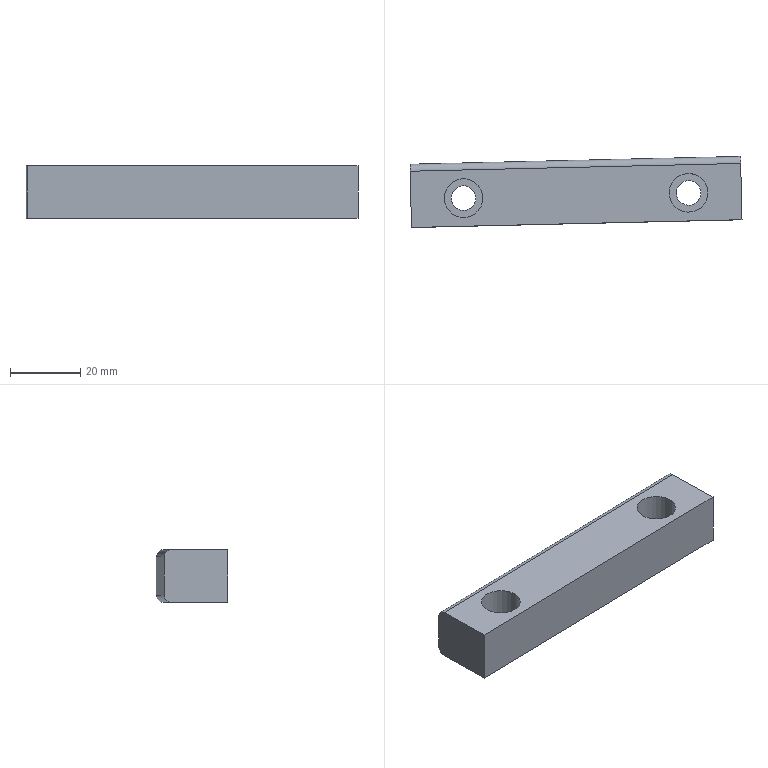Part | NX | features solid 2 | 1 solid | 14 faces | box 94.397 x 20.206 x 15 mm | volume 23046 mm3 | plane 8 | cylinder 6 | commonest cylinder face diameters 4 x2 7 x2 11 x2
STEP:
#1=CARTESIAN_POINT('',(641.92,-127.62,-12.));
#2=VERTEX_POINT('',#1);
#3=CARTESIAN_POINT('',(641.544,-111.625,-12.));
#4=VERTEX_POINT('',#3);
#5=CARTESIAN_POINT('',(641.732,-119.622,-12.));
#6=DIRECTION('',(-0.02352,0.9997,0.));
#7=VECTOR('',#6,1000.);
#8=LINE('',#5,#7);
#9=EDGE_CURVE('',#2,#4,#8,.T.);
#10=ORIENTED_EDGE('',*,*,#9,.T.);
#11=CARTESIAN_POINT('',(735.518,-109.413,-12.));
#12=VERTEX_POINT('',#11);
#13=CARTESIAN_POINT('',(735.518,-109.413,-12.));
#14=DIRECTION('',(0.9997,0.02352,0.));
#15=VECTOR('',#14,1000.);
#16=LINE('',#13,#15);
#17=EDGE_CURVE('',#4,#12,#16,.T.);
#18=ORIENTED_EDGE('',*,*,#17,.T.);
#19=CARTESIAN_POINT('',(735.894,-125.409,-12.));
#20=VERTEX_POINT('',#19);
#21=CARTESIAN_POINT('',(735.706,-117.411,-12.));
#22=DIRECTION('',(-0.02352,0.9997,0.));
#23=VECTOR('',#22,1000.);
#24=LINE('',#21,#23);
#25=EDGE_CURVE('',#20,#12,#24,.T.);
#26=ORIENTED_EDGE('',*,*,#25,.F.);
#27=CARTESIAN_POINT('',(735.894,-125.409,-12.));
#28=DIRECTION('',(0.9997,0.02352,0.));
#29=VECTOR('',#28,1000.);
#30=LINE('',#27,#29);
#31=EDGE_CURVE('',#2,#20,#30,.T.);
#32=ORIENTED_EDGE('',*,*,#31,.F.);
#33=EDGE_LOOP('',(#10,#18,#26,#32));
#34=FACE_BOUND('',#33,.T.);
#35=CARTESIAN_POINT('',(660.228,-119.27,-12.));
#36=VERTEX_POINT('',#35);
#37=CARTESIAN_POINT('',(656.728,-119.27,-12.));
#38=DIRECTION('',(0.,0.,1.));
#39=DIRECTION('',(1.,0.,0.));
#40=AXIS2_PLACEMENT_3D('',#37,#38,#39);
#41=CIRCLE('',#40,3.5);
#42=EDGE_CURVE('',#36,#36,#41,.T.);
#43=ORIENTED_EDGE('',*,*,#42,.T.);
#44=EDGE_LOOP('',(#43));
#45=FACE_BOUND('',#44,.T.);
#46=CARTESIAN_POINT('',(717.214,-117.929,-12.));
#47=VERTEX_POINT('',#46);
#48=CARTESIAN_POINT('',(720.71,-117.764,-12.));
#49=DIRECTION('',(0.,0.,-1.));
#50=DIRECTION('',(-0.9989,-0.04703,0.));
#51=AXIS2_PLACEMENT_3D('',#48,#49,#50);
#52=CIRCLE('',#51,3.5);
#53=EDGE_CURVE('',#47,#47,#52,.T.);
#54=ORIENTED_EDGE('',*,*,#53,.F.);
#55=EDGE_LOOP('',(#54));
#56=FACE_BOUND('',#55,.T.);
#57=CARTESIAN_POINT('',(735.706,-117.411,-12.));
#58=DIRECTION('',(0.,0.,1.));
#59=DIRECTION('',(1.,0.,0.));
#60=AXIS2_PLACEMENT_3D('',#57,#58,#59);
#61=PLANE('',#60);
#62=ADVANCED_FACE('',(#34,#45,#56),#61,.F.);
#63=CARTESIAN_POINT('',(735.894,-125.409,3.));
#64=VERTEX_POINT('',#63);
#65=CARTESIAN_POINT('',(735.518,-109.413,3.));
#66=VERTEX_POINT('',#65);
#67=CARTESIAN_POINT('',(735.706,-117.411,3.));
#68=DIRECTION('',(-0.02352,0.9997,0.));
#69=VECTOR('',#68,1000.);
#70=LINE('',#67,#69);
#71=EDGE_CURVE('',#64,#66,#70,.T.);
#72=ORIENTED_EDGE('',*,*,#71,.T.);
#73=CARTESIAN_POINT('',(641.544,-111.625,3.));
#74=VERTEX_POINT('',#73);
#75=CARTESIAN_POINT('',(735.518,-109.413,3.));
#76=DIRECTION('',(-0.9997,-0.02352,0.));
#77=VECTOR('',#76,1000.);
#78=LINE('',#75,#77);
#79=EDGE_CURVE('',#66,#74,#78,.T.);
#80=ORIENTED_EDGE('',*,*,#79,.T.);
#81=CARTESIAN_POINT('',(641.92,-127.62,3.));
#82=VERTEX_POINT('',#81);
#83=CARTESIAN_POINT('',(641.732,-119.622,3.));
#84=DIRECTION('',(-0.02352,0.9997,0.));
#85=VECTOR('',#84,1000.);
#86=LINE('',#83,#85);
#87=EDGE_CURVE('',#82,#74,#86,.T.);
#88=ORIENTED_EDGE('',*,*,#87,.F.);
#89=CARTESIAN_POINT('',(735.894,-125.409,3.));
#90=DIRECTION('',(-0.9997,-0.02352,0.));
#91=VECTOR('',#90,1000.);
#92=LINE('',#89,#91);
#93=EDGE_CURVE('',#64,#82,#92,.T.);
#94=ORIENTED_EDGE('',*,*,#93,.F.);
#95=EDGE_LOOP('',(#72,#80,#88,#94));
#96=FACE_BOUND('',#95,.T.);
#97=CARTESIAN_POINT('',(662.228,-119.27,3.));
#98=VERTEX_POINT('',#97);
#99=CARTESIAN_POINT('',(656.728,-119.27,3.));
#100=DIRECTION('',(0.,0.,-1.));
#101=DIRECTION('',(1.,0.,0.));
#102=AXIS2_PLACEMENT_3D('',#99,#100,#101);
#103=CIRCLE('',#102,5.5);
#104=EDGE_CURVE('',#98,#98,#103,.T.);
#105=ORIENTED_EDGE('',*,*,#104,.T.);
#106=EDGE_LOOP('',(#105));
#107=FACE_BOUND('',#106,.T.);
#108=CARTESIAN_POINT('',(715.216,-118.023,3.));
#109=VERTEX_POINT('',#108);
#110=CARTESIAN_POINT('',(720.71,-117.764,3.));
#111=DIRECTION('',(0.,0.,1.));
#112=DIRECTION('',(-0.9989,-0.04703,0.));
#113=AXIS2_PLACEMENT_3D('',#110,#111,#112);
#114=CIRCLE('',#113,5.5);
#115=EDGE_CURVE('',#109,#109,#114,.T.);
#116=ORIENTED_EDGE('',*,*,#115,.F.);
#117=EDGE_LOOP('',(#116));
#118=FACE_BOUND('',#117,.T.);
#119=CARTESIAN_POINT('',(735.706,-117.411,3.));
#120=DIRECTION('',(0.,0.,-1.));
#121=DIRECTION('',(-1.,0.,0.));
#122=AXIS2_PLACEMENT_3D('',#119,#120,#121);
#123=PLANE('',#122);
#124=ADVANCED_FACE('',(#96,#107,#118),#123,.F.);
#125=CARTESIAN_POINT('',(641.496,-109.625,1.));
#126=VERTEX_POINT('',#125);
#127=CARTESIAN_POINT('',(641.496,-109.625,-10.));
#128=VERTEX_POINT('',#127);
#129=CARTESIAN_POINT('',(641.496,-109.625,50.));
#130=DIRECTION('',(0.,0.,-1.));
#131=VECTOR('',#130,1000.);
#132=LINE('',#129,#131);
#133=EDGE_CURVE('',#126,#128,#132,.T.);
#134=ORIENTED_EDGE('',*,*,#133,.T.);
#135=CARTESIAN_POINT('',(641.544,-111.625,-10.));
#136=DIRECTION('',(0.9997,0.02352,0.));
#137=DIRECTION('',(-0.02352,0.9997,0.));
#138=AXIS2_PLACEMENT_3D('',#135,#136,#137);
#139=CIRCLE('',#138,2.);
#140=EDGE_CURVE('',#128,#4,#139,.F.);
#141=ORIENTED_EDGE('',*,*,#140,.T.);
#142=ORIENTED_EDGE('',*,*,#9,.F.);
#143=CARTESIAN_POINT('',(641.92,-127.62,50.));
#144=DIRECTION('',(0.,0.,-1.));
#145=VECTOR('',#144,1000.);
#146=LINE('',#143,#145);
#147=EDGE_CURVE('',#82,#2,#146,.T.);
#148=ORIENTED_EDGE('',*,*,#147,.F.);
#149=ORIENTED_EDGE('',*,*,#87,.T.);
#150=CARTESIAN_POINT('',(641.544,-111.625,1.));
#151=DIRECTION('',(0.9997,0.02352,0.));
#152=DIRECTION('',(-0.02352,0.9997,0.));
#153=AXIS2_PLACEMENT_3D('',#150,#151,#152);
#154=CIRCLE('',#153,2.);
#155=EDGE_CURVE('',#74,#126,#154,.F.);
#156=ORIENTED_EDGE('',*,*,#155,.T.);
#157=EDGE_LOOP('',(#134,#141,#142,#148,#149,#156));
#158=FACE_BOUND('',#157,.T.);
#159=CARTESIAN_POINT('',(641.732,-119.622,50.));
#160=DIRECTION('',(0.9997,0.02352,0.));
#161=DIRECTION('',(-0.02352,0.9997,0.));
#162=AXIS2_PLACEMENT_3D('',#159,#160,#161);
#163=PLANE('',#162);
#164=ADVANCED_FACE('',(#158),#163,.F.);
#165=ORIENTED_EDGE('',*,*,#25,.T.);
#166=CARTESIAN_POINT('',(735.47,-107.414,-10.));
#167=VERTEX_POINT('',#166);
#168=CARTESIAN_POINT('',(735.518,-109.413,-10.));
#169=DIRECTION('',(-0.9997,-0.02352,0.));
#170=DIRECTION('',(0.02352,-0.9997,0.));
#171=AXIS2_PLACEMENT_3D('',#168,#169,#170);
#172=CIRCLE('',#171,2.);
#173=EDGE_CURVE('',#12,#167,#172,.F.);
#174=ORIENTED_EDGE('',*,*,#173,.T.);
#175=CARTESIAN_POINT('',(735.47,-107.414,1.));
#176=VERTEX_POINT('',#175);
#177=CARTESIAN_POINT('',(735.47,-107.414,50.));
#178=DIRECTION('',(0.,0.,1.));
#179=VECTOR('',#178,1000.);
#180=LINE('',#177,#179);
#181=EDGE_CURVE('',#167,#176,#180,.T.);
#182=ORIENTED_EDGE('',*,*,#181,.T.);
#183=CARTESIAN_POINT('',(735.518,-109.413,1.));
#184=DIRECTION('',(-0.9997,-0.02352,0.));
#185=DIRECTION('',(0.02352,-0.9997,0.));
#186=AXIS2_PLACEMENT_3D('',#183,#184,#185);
#187=CIRCLE('',#186,2.);
#188=EDGE_CURVE('',#176,#66,#187,.F.);
#189=ORIENTED_EDGE('',*,*,#188,.T.);
#190=ORIENTED_EDGE('',*,*,#71,.F.);
#191=CARTESIAN_POINT('',(735.894,-125.409,50.));
#192=DIRECTION('',(0.,0.,1.));
#193=VECTOR('',#192,1000.);
#194=LINE('',#191,#193);
#195=EDGE_CURVE('',#20,#64,#194,.T.);
#196=ORIENTED_EDGE('',*,*,#195,.F.);
#197=EDGE_LOOP('',(#165,#174,#182,#189,#190,#196));
#198=FACE_BOUND('',#197,.T.);
#199=CARTESIAN_POINT('',(735.706,-117.411,50.));
#200=DIRECTION('',(-0.9997,-0.02352,0.));
#201=DIRECTION('',(0.02352,-0.9997,0.));
#202=AXIS2_PLACEMENT_3D('',#199,#200,#201);
#203=PLANE('',#202);
#204=ADVANCED_FACE('',(#198),#203,.F.);
#205=ORIENTED_EDGE('',*,*,#147,.T.);
#206=ORIENTED_EDGE('',*,*,#31,.T.);
#207=ORIENTED_EDGE('',*,*,#195,.T.);
#208=ORIENTED_EDGE('',*,*,#93,.T.);
#209=EDGE_LOOP('',(#205,#206,#207,#208));
#210=FACE_BOUND('',#209,.T.);
#211=CARTESIAN_POINT('',(735.894,-125.409,50.));
#212=DIRECTION('',(0.02352,-0.9997,0.));
#213=DIRECTION('',(0.9997,0.02352,0.));
#214=AXIS2_PLACEMENT_3D('',#211,#212,#213);
#215=PLANE('',#214);
#216=ADVANCED_FACE('',(#210),#215,.T.);
#217=ORIENTED_EDGE('',*,*,#181,.F.);
#218=CARTESIAN_POINT('',(735.47,-107.414,-10.));
#219=DIRECTION('',(0.9997,0.02352,0.));
#220=VECTOR('',#219,1000.);
#221=LINE('',#218,#220);
#222=EDGE_CURVE('',#167,#128,#221,.F.);
#223=ORIENTED_EDGE('',*,*,#222,.T.);
#224=ORIENTED_EDGE('',*,*,#133,.F.);
#225=CARTESIAN_POINT('',(735.47,-107.414,1.));
#226=DIRECTION('',(-0.9997,-0.02352,0.));
#227=VECTOR('',#226,1000.);
#228=LINE('',#225,#227);
#229=EDGE_CURVE('',#126,#176,#228,.F.);
#230=ORIENTED_EDGE('',*,*,#229,.T.);
#231=EDGE_LOOP('',(#217,#223,#224,#230));
#232=FACE_BOUND('',#231,.T.);
#233=CARTESIAN_POINT('',(735.47,-107.414,50.));
#234=DIRECTION('',(0.02352,-0.9997,0.));
#235=DIRECTION('',(0.9997,0.02352,0.));
#236=AXIS2_PLACEMENT_3D('',#233,#234,#235);
#237=PLANE('',#236);
#238=ADVANCED_FACE('',(#232),#237,.F.);
#239=ORIENTED_EDGE('',*,*,#140,.F.);
#240=ORIENTED_EDGE('',*,*,#222,.F.);
#241=ORIENTED_EDGE('',*,*,#173,.F.);
#242=ORIENTED_EDGE('',*,*,#17,.F.);
#243=EDGE_LOOP('',(#239,#240,#241,#242));
#244=FACE_BOUND('',#243,.T.);
#245=CARTESIAN_POINT('',(735.518,-109.413,-10.));
#246=DIRECTION('',(0.9997,0.02352,0.));
#247=DIRECTION('',(-0.02352,0.9997,0.));
#248=AXIS2_PLACEMENT_3D('',#245,#246,#247);
#249=CYLINDRICAL_SURFACE('',#248,2.);
#250=ADVANCED_FACE('',(#244),#249,.T.);
#251=ORIENTED_EDGE('',*,*,#188,.F.);
#252=ORIENTED_EDGE('',*,*,#229,.F.);
#253=ORIENTED_EDGE('',*,*,#155,.F.);
#254=ORIENTED_EDGE('',*,*,#79,.F.);
#255=EDGE_LOOP('',(#251,#252,#253,#254));
#256=FACE_BOUND('',#255,.T.);
#257=CARTESIAN_POINT('',(735.518,-109.413,1.));
#258=DIRECTION('',(-0.9997,-0.02352,0.));
#259=DIRECTION('',(0.02352,-0.9997,0.));
#260=AXIS2_PLACEMENT_3D('',#257,#258,#259);
#261=CYLINDRICAL_SURFACE('',#260,2.);
#262=ADVANCED_FACE('',(#256),#261,.T.);
#263=CARTESIAN_POINT('',(653.228,-119.27,-6.));
#264=VERTEX_POINT('',#263);
#265=CARTESIAN_POINT('',(656.728,-119.27,-6.));
#266=DIRECTION('',(0.,0.,-1.));
#267=DIRECTION('',(-1.,0.,0.));
#268=AXIS2_PLACEMENT_3D('',#265,#266,#267);
#269=CIRCLE('',#268,3.5);
#270=EDGE_CURVE('',#264,#264,#269,.T.);
#271=ORIENTED_EDGE('',*,*,#270,.F.);
#272=EDGE_LOOP('',(#271));
#273=FACE_BOUND('',#272,.T.);
#274=ORIENTED_EDGE('',*,*,#42,.F.);
#275=EDGE_LOOP('',(#274));
#276=FACE_BOUND('',#275,.T.);
#277=CARTESIAN_POINT('',(656.728,-119.27,3.));
#278=DIRECTION('',(0.,0.,-1.));
#279=DIRECTION('',(1.,0.,0.));
#280=AXIS2_PLACEMENT_3D('',#277,#278,#279);
#281=CYLINDRICAL_SURFACE('',#280,3.5);
#282=ADVANCED_FACE('',(#273,#276),#281,.F.);
#283=ORIENTED_EDGE('',*,*,#270,.T.);
#284=EDGE_LOOP('',(#283));
#285=FACE_BOUND('',#284,.T.);
#286=CARTESIAN_POINT('',(662.228,-119.27,-6.));
#287=VERTEX_POINT('',#286);
#288=CARTESIAN_POINT('',(656.728,-119.27,-6.));
#289=DIRECTION('',(0.,0.,1.));
#290=DIRECTION('',(1.,0.,0.));
#291=AXIS2_PLACEMENT_3D('',#288,#289,#290);
#292=CIRCLE('',#291,5.5);
#293=EDGE_CURVE('',#287,#287,#292,.F.);
#294=ORIENTED_EDGE('',*,*,#293,.F.);
#295=EDGE_LOOP('',(#294));
#296=FACE_BOUND('',#295,.T.);
#297=CARTESIAN_POINT('',(656.728,-119.27,-6.));
#298=DIRECTION('',(0.,0.,-1.));
#299=DIRECTION('',(-1.,0.,0.));
#300=AXIS2_PLACEMENT_3D('',#297,#298,#299);
#301=PLANE('',#300);
#302=ADVANCED_FACE('',(#285,#296),#301,.F.);
#303=ORIENTED_EDGE('',*,*,#293,.T.);
#304=EDGE_LOOP('',(#303));
#305=FACE_BOUND('',#304,.T.);
#306=ORIENTED_EDGE('',*,*,#104,.F.);
#307=EDGE_LOOP('',(#306));
#308=FACE_BOUND('',#307,.T.);
#309=CARTESIAN_POINT('',(656.728,-119.27,3.));
#310=DIRECTION('',(0.,0.,-1.));
#311=DIRECTION('',(1.,0.,0.));
#312=AXIS2_PLACEMENT_3D('',#309,#310,#311);
#313=CYLINDRICAL_SURFACE('',#312,5.5);
#314=ADVANCED_FACE('',(#305,#308),#313,.F.);
#315=CARTESIAN_POINT('',(724.206,-117.599,-6.));
#316=VERTEX_POINT('',#315);
#317=CARTESIAN_POINT('',(720.71,-117.764,-6.));
#318=DIRECTION('',(0.,0.,1.));
#319=DIRECTION('',(0.9989,0.04703,0.));
#320=AXIS2_PLACEMENT_3D('',#317,#318,#319);
#321=CIRCLE('',#320,3.5);
#322=EDGE_CURVE('',#316,#316,#321,.T.);
#323=ORIENTED_EDGE('',*,*,#322,.T.);
#324=EDGE_LOOP('',(#323));
#325=FACE_BOUND('',#324,.T.);
#326=ORIENTED_EDGE('',*,*,#53,.T.);
#327=EDGE_LOOP('',(#326));
#328=FACE_BOUND('',#327,.T.);
#329=CARTESIAN_POINT('',(720.71,-117.764,3.));
#330=DIRECTION('',(0.,0.,-1.));
#331=DIRECTION('',(-0.9989,-0.04703,0.));
#332=AXIS2_PLACEMENT_3D('',#329,#330,#331);
#333=CYLINDRICAL_SURFACE('',#332,3.5);
#334=ADVANCED_FACE('',(#325,#328),#333,.F.);
#335=ORIENTED_EDGE('',*,*,#322,.F.);
#336=EDGE_LOOP('',(#335));
#337=FACE_BOUND('',#336,.T.);
#338=CARTESIAN_POINT('',(715.216,-118.023,-6.));
#339=VERTEX_POINT('',#338);
#340=CARTESIAN_POINT('',(720.71,-117.764,-6.));
#341=DIRECTION('',(0.,0.,-1.));
#342=DIRECTION('',(-0.9989,-0.04703,0.));
#343=AXIS2_PLACEMENT_3D('',#340,#341,#342);
#344=CIRCLE('',#343,5.5);
#345=EDGE_CURVE('',#339,#339,#344,.F.);
#346=ORIENTED_EDGE('',*,*,#345,.T.);
#347=EDGE_LOOP('',(#346));
#348=FACE_BOUND('',#347,.T.);
#349=CARTESIAN_POINT('',(720.71,-117.764,-6.));
#350=DIRECTION('',(0.,0.,-1.));
#351=DIRECTION('',(0.9989,0.04703,0.));
#352=AXIS2_PLACEMENT_3D('',#349,#350,#351);
#353=PLANE('',#352);
#354=ADVANCED_FACE('',(#337,#348),#353,.F.);
#355=ORIENTED_EDGE('',*,*,#345,.F.);
#356=EDGE_LOOP('',(#355));
#357=FACE_BOUND('',#356,.T.);
#358=ORIENTED_EDGE('',*,*,#115,.T.);
#359=EDGE_LOOP('',(#358));
#360=FACE_BOUND('',#359,.T.);
#361=CARTESIAN_POINT('',(720.71,-117.764,3.));
#362=DIRECTION('',(0.,0.,-1.));
#363=DIRECTION('',(-0.9989,-0.04703,0.));
#364=AXIS2_PLACEMENT_3D('',#361,#362,#363);
#365=CYLINDRICAL_SURFACE('',#364,5.5);
#366=ADVANCED_FACE('',(#357,#360),#365,.F.);
#367=CLOSED_SHELL('',(#62,#124,#164,#204,#216,#238,#250,#262,#282,#302,#314,#334,#354,#366));
#368=MANIFOLD_SOLID_BREP('',#367);
#369=(LENGTH_UNIT()NAMED_UNIT(*)SI_UNIT(.MILLI.,.METRE.));
#370=UNCERTAINTY_MEASURE_WITH_UNIT(LENGTH_MEASURE(0.00001),#369,'','');
#371=(NAMED_UNIT(*)PLANE_ANGLE_UNIT()SI_UNIT($,.RADIAN.));
#372=(NAMED_UNIT(*)SI_UNIT($,.STERADIAN.)SOLID_ANGLE_UNIT());
#373=(GEOMETRIC_REPRESENTATION_CONTEXT(3)GLOBAL_UNCERTAINTY_ASSIGNED_CONTEXT((#370))GLOBAL_UNIT_ASSIGNED_CONTEXT((#369,#371,#372))REPRESENTATION_CONTEXT('',''));
#374=ADVANCED_BREP_SHAPE_REPRESENTATION('',(#368),#373);